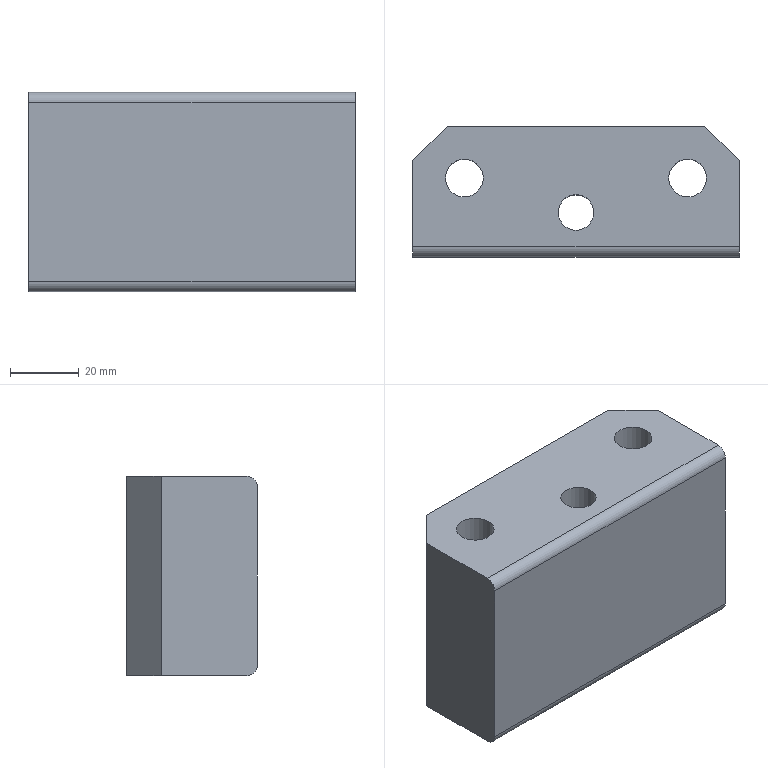Part | NX | features solid 2 | 1 solid | 19 faces | box 95 x 38 x 58 mm | volume 171870 mm3 | plane 11 | cylinder 8 | commonest cylinder face diameters 17 x3 6 x2 11 x2 10.3 x1
STEP:
#1=CARTESIAN_POINT('',(2412.5,497.,123.));
#2=VERTEX_POINT('',#1);
#3=CARTESIAN_POINT('',(2412.5,497.,71.));
#4=VERTEX_POINT('',#3);
#5=CARTESIAN_POINT('',(2412.5,497.,-60.));
#6=DIRECTION('',(0.,0.,-1.));
#7=VECTOR('',#6,1000.);
#8=LINE('',#5,#7);
#9=EDGE_CURVE('',#2,#4,#8,.T.);
#10=ORIENTED_EDGE('',*,*,#9,.T.);
#11=CARTESIAN_POINT('',(2507.5,497.,71.));
#12=VERTEX_POINT('',#11);
#13=CARTESIAN_POINT('',(2407.5,497.,71.));
#14=DIRECTION('',(1.,0.,0.));
#15=VECTOR('',#14,1000.);
#16=LINE('',#13,#15);
#17=EDGE_CURVE('',#4,#12,#16,.T.);
#18=ORIENTED_EDGE('',*,*,#17,.T.);
#19=CARTESIAN_POINT('',(2507.5,497.,123.));
#20=VERTEX_POINT('',#19);
#21=CARTESIAN_POINT('',(2507.5,497.,52.5));
#22=DIRECTION('',(0.,0.,1.));
#23=VECTOR('',#22,1000.);
#24=LINE('',#21,#23);
#25=EDGE_CURVE('',#12,#20,#24,.T.);
#26=ORIENTED_EDGE('',*,*,#25,.T.);
#27=CARTESIAN_POINT('',(2437.,497.,123.));
#28=DIRECTION('',(-1.,0.,0.));
#29=VECTOR('',#28,1000.);
#30=LINE('',#27,#29);
#31=EDGE_CURVE('',#20,#2,#30,.T.);
#32=ORIENTED_EDGE('',*,*,#31,.T.);
#33=EDGE_LOOP('',(#10,#18,#26,#32));
#34=FACE_BOUND('',#33,.T.);
#35=CARTESIAN_POINT('',(2437.,497.,99.));
#36=DIRECTION('',(0.,1.,0.));
#37=DIRECTION('',(0.,0.,1.));
#38=AXIS2_PLACEMENT_3D('',#35,#36,#37);
#39=PLANE('',#38);
#40=ADVANCED_FACE('',(#34),#39,.F.);
#41=CARTESIAN_POINT('',(2427.5,525.5,106.));
#42=VERTEX_POINT('',#41);
#43=CARTESIAN_POINT('',(2427.5,520.,106.));
#44=DIRECTION('',(0.,0.,-1.));
#45=DIRECTION('',(0.,1.,0.));
#46=AXIS2_PLACEMENT_3D('',#43,#44,#45);
#47=CIRCLE('',#46,5.5);
#48=EDGE_CURVE('',#42,#42,#47,.T.);
#49=ORIENTED_EDGE('',*,*,#48,.F.);
#50=EDGE_LOOP('',(#49));
#51=FACE_BOUND('',#50,.T.);
#52=CARTESIAN_POINT('',(2427.5,528.5,106.));
#53=VERTEX_POINT('',#52);
#54=CARTESIAN_POINT('',(2427.5,520.,106.));
#55=DIRECTION('',(0.,0.,-1.));
#56=DIRECTION('',(0.,1.,0.));
#57=AXIS2_PLACEMENT_3D('',#54,#55,#56);
#58=CIRCLE('',#57,8.5);
#59=EDGE_CURVE('',#53,#53,#58,.T.);
#60=ORIENTED_EDGE('',*,*,#59,.T.);
#61=EDGE_LOOP('',(#60));
#62=FACE_BOUND('',#61,.T.);
#63=CARTESIAN_POINT('',(1913.818,1175.578,106.));
#64=DIRECTION('',(0.,0.,1.));
#65=DIRECTION('',(0.,1.,0.));
#66=AXIS2_PLACEMENT_3D('',#63,#64,#65);
#67=PLANE('',#66);
#68=ADVANCED_FACE('',(#51,#62),#67,.F.);
#69=CARTESIAN_POINT('',(2492.5,525.5,106.));
#70=VERTEX_POINT('',#69);
#71=CARTESIAN_POINT('',(2492.5,520.,106.));
#72=DIRECTION('',(0.,0.,-1.));
#73=DIRECTION('',(0.,1.,0.));
#74=AXIS2_PLACEMENT_3D('',#71,#72,#73);
#75=CIRCLE('',#74,5.5);
#76=EDGE_CURVE('',#70,#70,#75,.T.);
#77=ORIENTED_EDGE('',*,*,#76,.F.);
#78=EDGE_LOOP('',(#77));
#79=FACE_BOUND('',#78,.T.);
#80=CARTESIAN_POINT('',(2492.5,528.5,106.));
#81=VERTEX_POINT('',#80);
#82=CARTESIAN_POINT('',(2492.5,520.,106.));
#83=DIRECTION('',(0.,0.,-1.));
#84=DIRECTION('',(0.,1.,0.));
#85=AXIS2_PLACEMENT_3D('',#82,#83,#84);
#86=CIRCLE('',#85,8.5);
#87=EDGE_CURVE('',#81,#81,#86,.T.);
#88=ORIENTED_EDGE('',*,*,#87,.T.);
#89=EDGE_LOOP('',(#88));
#90=FACE_BOUND('',#89,.T.);
#91=CARTESIAN_POINT('',(1906.818,1177.578,106.));
#92=DIRECTION('',(0.,0.,1.));
#93=DIRECTION('',(0.,1.,0.));
#94=AXIS2_PLACEMENT_3D('',#91,#92,#93);
#95=PLANE('',#94);
#96=ADVANCED_FACE('',(#79,#90),#95,.F.);
#97=CARTESIAN_POINT('',(2412.5,500.,68.));
#98=VERTEX_POINT('',#97);
#99=CARTESIAN_POINT('',(2412.5,500.,71.));
#100=DIRECTION('',(-1.,0.,0.));
#101=DIRECTION('',(0.,1.,0.));
#102=AXIS2_PLACEMENT_3D('',#99,#100,#101);
#103=CIRCLE('',#102,3.);
#104=EDGE_CURVE('',#98,#4,#103,.T.);
#105=ORIENTED_EDGE('',*,*,#104,.F.);
#106=CARTESIAN_POINT('',(2507.5,500.,68.));
#107=VERTEX_POINT('',#106);
#108=CARTESIAN_POINT('',(2467.5,500.,68.));
#109=DIRECTION('',(-1.,0.,0.));
#110=VECTOR('',#109,1000.);
#111=LINE('',#108,#110);
#112=EDGE_CURVE('',#107,#98,#111,.T.);
#113=ORIENTED_EDGE('',*,*,#112,.F.);
#114=CARTESIAN_POINT('',(2507.5,500.,71.));
#115=DIRECTION('',(-1.,0.,0.));
#116=DIRECTION('',(0.,0.,1.));
#117=AXIS2_PLACEMENT_3D('',#114,#115,#116);
#118=CIRCLE('',#117,3.);
#119=EDGE_CURVE('',#107,#12,#118,.T.);
#120=ORIENTED_EDGE('',*,*,#119,.T.);
#121=ORIENTED_EDGE('',*,*,#17,.F.);
#122=EDGE_LOOP('',(#105,#113,#120,#121));
#123=FACE_BOUND('',#122,.T.);
#124=CARTESIAN_POINT('',(1911.818,500.,71.));
#125=DIRECTION('',(1.,0.,0.));
#126=DIRECTION('',(0.,0.,1.));
#127=AXIS2_PLACEMENT_3D('',#124,#125,#126);
#128=CYLINDRICAL_SURFACE('',#127,3.);
#129=ADVANCED_FACE('',(#123),#128,.T.);
#130=CARTESIAN_POINT('',(2412.5,525.,68.));
#131=VERTEX_POINT('',#130);
#132=CARTESIAN_POINT('',(2412.5,390.,68.));
#133=DIRECTION('',(0.,-1.,0.));
#134=VECTOR('',#133,1000.);
#135=LINE('',#132,#134);
#136=EDGE_CURVE('',#131,#98,#135,.T.);
#137=ORIENTED_EDGE('',*,*,#136,.T.);
#138=ORIENTED_EDGE('',*,*,#104,.T.);
#139=ORIENTED_EDGE('',*,*,#9,.F.);
#140=CARTESIAN_POINT('',(2412.5,500.,126.));
#141=VERTEX_POINT('',#140);
#142=CARTESIAN_POINT('',(2412.5,500.,123.));
#143=DIRECTION('',(-1.,0.,0.));
#144=DIRECTION('',(0.,1.,0.));
#145=AXIS2_PLACEMENT_3D('',#142,#143,#144);
#146=CIRCLE('',#145,3.);
#147=EDGE_CURVE('',#2,#141,#146,.T.);
#148=ORIENTED_EDGE('',*,*,#147,.T.);
#149=CARTESIAN_POINT('',(2412.5,525.,126.));
#150=VERTEX_POINT('',#149);
#151=CARTESIAN_POINT('',(2412.5,390.,126.));
#152=DIRECTION('',(0.,1.,0.));
#153=VECTOR('',#152,1000.);
#154=LINE('',#151,#153);
#155=EDGE_CURVE('',#141,#150,#154,.T.);
#156=ORIENTED_EDGE('',*,*,#155,.T.);
#157=CARTESIAN_POINT('',(2412.5,525.,-60.));
#158=DIRECTION('',(0.,0.,-1.));
#159=VECTOR('',#158,1000.);
#160=LINE('',#157,#159);
#161=EDGE_CURVE('',#150,#131,#160,.T.);
#162=ORIENTED_EDGE('',*,*,#161,.T.);
#163=EDGE_LOOP('',(#137,#138,#139,#148,#156,#162));
#164=FACE_BOUND('',#163,.T.);
#165=CARTESIAN_POINT('',(2412.5,390.,-60.));
#166=DIRECTION('',(1.,0.,0.));
#167=DIRECTION('',(0.,1.,0.));
#168=AXIS2_PLACEMENT_3D('',#165,#166,#167);
#169=PLANE('',#168);
#170=ADVANCED_FACE('',(#164),#169,.F.);
#171=CARTESIAN_POINT('',(2422.5,535.,126.));
#172=VERTEX_POINT('',#171);
#173=CARTESIAN_POINT('',(2490.948,603.448,126.));
#174=DIRECTION('',(-0.7071,-0.7071,0.));
#175=VECTOR('',#174,1000.);
#176=LINE('',#173,#175);
#177=EDGE_CURVE('',#172,#150,#176,.T.);
#178=ORIENTED_EDGE('',*,*,#177,.F.);
#179=CARTESIAN_POINT('',(2422.5,535.,68.));
#180=VERTEX_POINT('',#179);
#181=CARTESIAN_POINT('',(2422.5,535.,52.5));
#182=DIRECTION('',(0.,0.,1.));
#183=VECTOR('',#182,1000.);
#184=LINE('',#181,#183);
#185=EDGE_CURVE('',#180,#172,#184,.T.);
#186=ORIENTED_EDGE('',*,*,#185,.F.);
#187=CARTESIAN_POINT('',(2490.948,603.448,68.));
#188=DIRECTION('',(0.7071,0.7071,0.));
#189=VECTOR('',#188,1000.);
#190=LINE('',#187,#189);
#191=EDGE_CURVE('',#131,#180,#190,.T.);
#192=ORIENTED_EDGE('',*,*,#191,.F.);
#193=ORIENTED_EDGE('',*,*,#161,.F.);
#194=EDGE_LOOP('',(#178,#186,#192,#193));
#195=FACE_BOUND('',#194,.T.);
#196=CARTESIAN_POINT('',(2422.5,535.,52.5));
#197=DIRECTION('',(-0.7071,0.7071,0.));
#198=DIRECTION('',(0.,0.,-1.));
#199=AXIS2_PLACEMENT_3D('',#196,#197,#198);
#200=PLANE('',#199);
#201=ADVANCED_FACE('',(#195),#200,.T.);
#202=CARTESIAN_POINT('',(2497.5,535.,126.));
#203=VERTEX_POINT('',#202);
#204=CARTESIAN_POINT('',(2435.,535.,126.));
#205=DIRECTION('',(1.,0.,0.));
#206=VECTOR('',#205,1000.);
#207=LINE('',#204,#206);
#208=EDGE_CURVE('',#172,#203,#207,.T.);
#209=ORIENTED_EDGE('',*,*,#208,.T.);
#210=CARTESIAN_POINT('',(2497.5,535.,68.));
#211=VERTEX_POINT('',#210);
#212=CARTESIAN_POINT('',(2497.5,535.,52.5));
#213=DIRECTION('',(0.,0.,-1.));
#214=VECTOR('',#213,1000.);
#215=LINE('',#212,#214);
#216=EDGE_CURVE('',#203,#211,#215,.T.);
#217=ORIENTED_EDGE('',*,*,#216,.T.);
#218=CARTESIAN_POINT('',(2435.,535.,68.));
#219=DIRECTION('',(-1.,0.,0.));
#220=VECTOR('',#219,1000.);
#221=LINE('',#218,#220);
#222=EDGE_CURVE('',#211,#180,#221,.T.);
#223=ORIENTED_EDGE('',*,*,#222,.T.);
#224=ORIENTED_EDGE('',*,*,#185,.T.);
#225=EDGE_LOOP('',(#209,#217,#223,#224));
#226=FACE_BOUND('',#225,.T.);
#227=CARTESIAN_POINT('',(2435.,535.,52.5));
#228=DIRECTION('',(0.,1.,0.));
#229=DIRECTION('',(0.,0.,1.));
#230=AXIS2_PLACEMENT_3D('',#227,#228,#229);
#231=PLANE('',#230);
#232=ADVANCED_FACE('',(#226),#231,.T.);
#233=CARTESIAN_POINT('',(2507.5,525.,126.));
#234=VERTEX_POINT('',#233);
#235=CARTESIAN_POINT('',(1880.87,1151.63,126.));
#236=DIRECTION('',(-0.7071,0.7071,0.));
#237=VECTOR('',#236,1000.);
#238=LINE('',#235,#237);
#239=EDGE_CURVE('',#234,#203,#238,.T.);
#240=ORIENTED_EDGE('',*,*,#239,.F.);
#241=CARTESIAN_POINT('',(2507.5,525.,68.));
#242=VERTEX_POINT('',#241);
#243=CARTESIAN_POINT('',(2507.5,525.,52.5));
#244=DIRECTION('',(0.,0.,1.));
#245=VECTOR('',#244,1000.);
#246=LINE('',#243,#245);
#247=EDGE_CURVE('',#242,#234,#246,.T.);
#248=ORIENTED_EDGE('',*,*,#247,.F.);
#249=CARTESIAN_POINT('',(1880.87,1151.63,68.));
#250=DIRECTION('',(0.7071,-0.7071,0.));
#251=VECTOR('',#250,1000.);
#252=LINE('',#249,#251);
#253=EDGE_CURVE('',#211,#242,#252,.T.);
#254=ORIENTED_EDGE('',*,*,#253,.F.);
#255=ORIENTED_EDGE('',*,*,#216,.F.);
#256=EDGE_LOOP('',(#240,#248,#254,#255));
#257=FACE_BOUND('',#256,.T.);
#258=CARTESIAN_POINT('',(2507.5,525.,52.5));
#259=DIRECTION('',(-0.7071,-0.7071,0.));
#260=DIRECTION('',(0.,0.,1.));
#261=AXIS2_PLACEMENT_3D('',#258,#259,#260);
#262=PLANE('',#261);
#263=ADVANCED_FACE('',(#257),#262,.F.);
#264=CARTESIAN_POINT('',(2507.5,500.,126.));
#265=VERTEX_POINT('',#264);
#266=CARTESIAN_POINT('',(2507.5,500.,123.));
#267=DIRECTION('',(1.,0.,0.));
#268=DIRECTION('',(0.,0.,1.));
#269=AXIS2_PLACEMENT_3D('',#266,#267,#268);
#270=CIRCLE('',#269,3.);
#271=EDGE_CURVE('',#265,#20,#270,.T.);
#272=ORIENTED_EDGE('',*,*,#271,.T.);
#273=ORIENTED_EDGE('',*,*,#25,.F.);
#274=ORIENTED_EDGE('',*,*,#119,.F.);
#275=CARTESIAN_POINT('',(2507.5,440.,68.));
#276=DIRECTION('',(0.,1.,0.));
#277=VECTOR('',#276,1000.);
#278=LINE('',#275,#277);
#279=EDGE_CURVE('',#107,#242,#278,.T.);
#280=ORIENTED_EDGE('',*,*,#279,.T.);
#281=ORIENTED_EDGE('',*,*,#247,.T.);
#282=CARTESIAN_POINT('',(2507.5,440.,126.));
#283=DIRECTION('',(0.,-1.,0.));
#284=VECTOR('',#283,1000.);
#285=LINE('',#282,#284);
#286=EDGE_CURVE('',#234,#265,#285,.T.);
#287=ORIENTED_EDGE('',*,*,#286,.T.);
#288=EDGE_LOOP('',(#272,#273,#274,#280,#281,#287));
#289=FACE_BOUND('',#288,.T.);
#290=CARTESIAN_POINT('',(2507.5,440.,52.5));
#291=DIRECTION('',(1.,0.,0.));
#292=DIRECTION('',(0.,0.,1.));
#293=AXIS2_PLACEMENT_3D('',#290,#291,#292);
#294=PLANE('',#293);
#295=ADVANCED_FACE('',(#289),#294,.T.);
#296=ORIENTED_EDGE('',*,*,#147,.F.);
#297=ORIENTED_EDGE('',*,*,#31,.F.);
#298=ORIENTED_EDGE('',*,*,#271,.F.);
#299=CARTESIAN_POINT('',(2407.5,500.,126.));
#300=DIRECTION('',(1.,0.,0.));
#301=VECTOR('',#300,1000.);
#302=LINE('',#299,#301);
#303=EDGE_CURVE('',#141,#265,#302,.T.);
#304=ORIENTED_EDGE('',*,*,#303,.F.);
#305=EDGE_LOOP('',(#296,#297,#298,#304));
#306=FACE_BOUND('',#305,.T.);
#307=CARTESIAN_POINT('',(2437.,500.,123.));
#308=DIRECTION('',(-1.,0.,0.));
#309=DIRECTION('',(0.,0.,-1.));
#310=AXIS2_PLACEMENT_3D('',#307,#308,#309);
#311=CYLINDRICAL_SURFACE('',#310,3.);
#312=ADVANCED_FACE('',(#306),#311,.T.);
#313=CARTESIAN_POINT('',(2427.5,525.5,126.));
#314=VERTEX_POINT('',#313);
#315=CARTESIAN_POINT('',(2427.5,520.,126.));
#316=DIRECTION('',(0.,0.,1.));
#317=DIRECTION('',(0.,1.,0.));
#318=AXIS2_PLACEMENT_3D('',#315,#316,#317);
#319=CIRCLE('',#318,5.5);
#320=EDGE_CURVE('',#314,#314,#319,.T.);
#321=ORIENTED_EDGE('',*,*,#320,.T.);
#322=EDGE_LOOP('',(#321));
#323=FACE_BOUND('',#322,.T.);
#324=ORIENTED_EDGE('',*,*,#48,.T.);
#325=EDGE_LOOP('',(#324));
#326=FACE_BOUND('',#325,.T.);
#327=CARTESIAN_POINT('',(2427.5,520.,566.));
#328=DIRECTION('',(0.,0.,1.));
#329=DIRECTION('',(0.,-1.,0.));
#330=AXIS2_PLACEMENT_3D('',#327,#328,#329);
#331=CYLINDRICAL_SURFACE('',#330,5.5);
#332=ADVANCED_FACE('',(#323,#326),#331,.F.);
#333=CARTESIAN_POINT('',(2492.5,525.5,126.));
#334=VERTEX_POINT('',#333);
#335=CARTESIAN_POINT('',(2492.5,520.,126.));
#336=DIRECTION('',(0.,0.,1.));
#337=DIRECTION('',(0.,1.,0.));
#338=AXIS2_PLACEMENT_3D('',#335,#336,#337);
#339=CIRCLE('',#338,5.5);
#340=EDGE_CURVE('',#334,#334,#339,.T.);
#341=ORIENTED_EDGE('',*,*,#340,.T.);
#342=EDGE_LOOP('',(#341));
#343=FACE_BOUND('',#342,.T.);
#344=ORIENTED_EDGE('',*,*,#76,.T.);
#345=EDGE_LOOP('',(#344));
#346=FACE_BOUND('',#345,.T.);
#347=CARTESIAN_POINT('',(2492.5,520.,566.));
#348=DIRECTION('',(0.,0.,1.));
#349=DIRECTION('',(0.,-1.,0.));
#350=AXIS2_PLACEMENT_3D('',#347,#348,#349);
#351=CYLINDRICAL_SURFACE('',#350,5.5);
#352=ADVANCED_FACE('',(#343,#346),#351,.F.);
#353=CARTESIAN_POINT('',(2454.85,510.,126.));
#354=VERTEX_POINT('',#353);
#355=CARTESIAN_POINT('',(2460.,510.,126.));
#356=DIRECTION('',(0.,0.,-1.));
#357=DIRECTION('',(-1.,0.,0.));
#358=AXIS2_PLACEMENT_3D('',#355,#356,#357);
#359=CIRCLE('',#358,5.15);
#360=EDGE_CURVE('',#354,#354,#359,.T.);
#361=ORIENTED_EDGE('',*,*,#360,.T.);
#362=EDGE_LOOP('',(#361));
#363=FACE_BOUND('',#362,.T.);
#364=ORIENTED_EDGE('',*,*,#340,.F.);
#365=EDGE_LOOP('',(#364));
#366=FACE_BOUND('',#365,.T.);
#367=ORIENTED_EDGE('',*,*,#320,.F.);
#368=EDGE_LOOP('',(#367));
#369=FACE_BOUND('',#368,.T.);
#370=ORIENTED_EDGE('',*,*,#303,.T.);
#371=ORIENTED_EDGE('',*,*,#286,.F.);
#372=ORIENTED_EDGE('',*,*,#239,.T.);
#373=ORIENTED_EDGE('',*,*,#208,.F.);
#374=ORIENTED_EDGE('',*,*,#177,.T.);
#375=ORIENTED_EDGE('',*,*,#155,.F.);
#376=EDGE_LOOP('',(#370,#371,#372,#373,#374,#375));
#377=FACE_BOUND('',#376,.T.);
#378=CARTESIAN_POINT('',(1911.818,1177.578,126.));
#379=DIRECTION('',(0.,0.,1.));
#380=DIRECTION('',(0.,1.,0.));
#381=AXIS2_PLACEMENT_3D('',#378,#379,#380);
#382=PLANE('',#381);
#383=ADVANCED_FACE('',(#363,#366,#369,#377),#382,.T.);
#384=ORIENTED_EDGE('',*,*,#59,.F.);
#385=EDGE_LOOP('',(#384));
#386=FACE_BOUND('',#385,.T.);
#387=CARTESIAN_POINT('',(2427.5,528.5,68.));
#388=VERTEX_POINT('',#387);
#389=CARTESIAN_POINT('',(2427.5,520.,68.));
#390=DIRECTION('',(0.,0.,1.));
#391=DIRECTION('',(0.,1.,0.));
#392=AXIS2_PLACEMENT_3D('',#389,#390,#391);
#393=CIRCLE('',#392,8.5);
#394=EDGE_CURVE('',#388,#388,#393,.T.);
#395=ORIENTED_EDGE('',*,*,#394,.F.);
#396=EDGE_LOOP('',(#395));
#397=FACE_BOUND('',#396,.T.);
#398=CARTESIAN_POINT('',(2427.5,520.,48.));
#399=DIRECTION('',(0.,0.,1.));
#400=DIRECTION('',(0.,-1.,0.));
#401=AXIS2_PLACEMENT_3D('',#398,#399,#400);
#402=CYLINDRICAL_SURFACE('',#401,8.5);
#403=ADVANCED_FACE('',(#386,#397),#402,.F.);
#404=ORIENTED_EDGE('',*,*,#87,.F.);
#405=EDGE_LOOP('',(#404));
#406=FACE_BOUND('',#405,.T.);
#407=CARTESIAN_POINT('',(2492.5,528.5,68.));
#408=VERTEX_POINT('',#407);
#409=CARTESIAN_POINT('',(2492.5,520.,68.));
#410=DIRECTION('',(0.,0.,1.));
#411=DIRECTION('',(0.,1.,0.));
#412=AXIS2_PLACEMENT_3D('',#409,#410,#411);
#413=CIRCLE('',#412,8.5);
#414=EDGE_CURVE('',#408,#408,#413,.T.);
#415=ORIENTED_EDGE('',*,*,#414,.F.);
#416=EDGE_LOOP('',(#415));
#417=FACE_BOUND('',#416,.T.);
#418=CARTESIAN_POINT('',(2492.5,520.,48.));
#419=DIRECTION('',(0.,0.,1.));
#420=DIRECTION('',(0.,-1.,0.));
#421=AXIS2_PLACEMENT_3D('',#418,#419,#420);
#422=CYLINDRICAL_SURFACE('',#421,8.5);
#423=ADVANCED_FACE('',(#406,#417),#422,.F.);
#424=CARTESIAN_POINT('',(2460.,518.5,68.));
#425=VERTEX_POINT('',#424);
#426=CARTESIAN_POINT('',(2460.,510.,68.));
#427=DIRECTION('',(0.,0.,1.));
#428=DIRECTION('',(0.,1.,0.));
#429=AXIS2_PLACEMENT_3D('',#426,#427,#428);
#430=CIRCLE('',#429,8.5);
#431=EDGE_CURVE('',#425,#425,#430,.T.);
#432=ORIENTED_EDGE('',*,*,#431,.T.);
#433=EDGE_LOOP('',(#432));
#434=FACE_BOUND('',#433,.T.);
#435=ORIENTED_EDGE('',*,*,#414,.T.);
#436=EDGE_LOOP('',(#435));
#437=FACE_BOUND('',#436,.T.);
#438=ORIENTED_EDGE('',*,*,#394,.T.);
#439=EDGE_LOOP('',(#438));
#440=FACE_BOUND('',#439,.T.);
#441=ORIENTED_EDGE('',*,*,#279,.F.);
#442=ORIENTED_EDGE('',*,*,#112,.T.);
#443=ORIENTED_EDGE('',*,*,#136,.F.);
#444=ORIENTED_EDGE('',*,*,#191,.T.);
#445=ORIENTED_EDGE('',*,*,#222,.F.);
#446=ORIENTED_EDGE('',*,*,#253,.T.);
#447=EDGE_LOOP('',(#441,#442,#443,#444,#445,#446));
#448=FACE_BOUND('',#447,.T.);
#449=CARTESIAN_POINT('',(1911.818,1177.578,68.));
#450=DIRECTION('',(0.,0.,1.));
#451=DIRECTION('',(0.,1.,0.));
#452=AXIS2_PLACEMENT_3D('',#449,#450,#451);
#453=PLANE('',#452);
#454=ADVANCED_FACE('',(#434,#437,#440,#448),#453,.F.);
#455=CARTESIAN_POINT('',(2454.85,510.,106.));
#456=VERTEX_POINT('',#455);
#457=CARTESIAN_POINT('',(2460.,510.,106.));
#458=DIRECTION('',(0.,0.,-1.));
#459=DIRECTION('',(-1.,0.,0.));
#460=AXIS2_PLACEMENT_3D('',#457,#458,#459);
#461=CIRCLE('',#460,5.15);
#462=EDGE_CURVE('',#456,#456,#461,.T.);
#463=ORIENTED_EDGE('',*,*,#462,.F.);
#464=EDGE_LOOP('',(#463));
#465=FACE_BOUND('',#464,.T.);
#466=CARTESIAN_POINT('',(2460.,518.5,106.));
#467=VERTEX_POINT('',#466);
#468=CARTESIAN_POINT('',(2460.,510.,106.));
#469=DIRECTION('',(0.,0.,-1.));
#470=DIRECTION('',(0.,1.,0.));
#471=AXIS2_PLACEMENT_3D('',#468,#469,#470);
#472=CIRCLE('',#471,8.5);
#473=EDGE_CURVE('',#467,#467,#472,.T.);
#474=ORIENTED_EDGE('',*,*,#473,.T.);
#475=EDGE_LOOP('',(#474));
#476=FACE_BOUND('',#475,.T.);
#477=CARTESIAN_POINT('',(1874.318,1167.578,106.));
#478=DIRECTION('',(0.,0.,1.));
#479=DIRECTION('',(0.,1.,0.));
#480=AXIS2_PLACEMENT_3D('',#477,#478,#479);
#481=PLANE('',#480);
#482=ADVANCED_FACE('',(#465,#476),#481,.F.);
#483=ORIENTED_EDGE('',*,*,#360,.F.);
#484=EDGE_LOOP('',(#483));
#485=FACE_BOUND('',#484,.T.);
#486=ORIENTED_EDGE('',*,*,#462,.T.);
#487=EDGE_LOOP('',(#486));
#488=FACE_BOUND('',#487,.T.);
#489=CARTESIAN_POINT('',(2460.,510.,566.));
#490=DIRECTION('',(0.,0.,1.));
#491=DIRECTION('',(0.,-1.,0.));
#492=AXIS2_PLACEMENT_3D('',#489,#490,#491);
#493=CYLINDRICAL_SURFACE('',#492,5.15);
#494=ADVANCED_FACE('',(#485,#488),#493,.F.);
#495=ORIENTED_EDGE('',*,*,#473,.F.);
#496=EDGE_LOOP('',(#495));
#497=FACE_BOUND('',#496,.T.);
#498=ORIENTED_EDGE('',*,*,#431,.F.);
#499=EDGE_LOOP('',(#498));
#500=FACE_BOUND('',#499,.T.);
#501=CARTESIAN_POINT('',(2460.,510.,48.));
#502=DIRECTION('',(0.,0.,1.));
#503=DIRECTION('',(0.,-1.,0.));
#504=AXIS2_PLACEMENT_3D('',#501,#502,#503);
#505=CYLINDRICAL_SURFACE('',#504,8.5);
#506=ADVANCED_FACE('',(#497,#500),#505,.F.);
#507=CLOSED_SHELL('',(#40,#68,#96,#129,#170,#201,#232,#263,#295,#312,#332,#352,#383,#403,#423,#454,#482,#494,#506));
#508=MANIFOLD_SOLID_BREP('',#507);
#509=(LENGTH_UNIT()NAMED_UNIT(*)SI_UNIT(.MILLI.,.METRE.));
#510=UNCERTAINTY_MEASURE_WITH_UNIT(LENGTH_MEASURE(0.00001),#509,'','');
#511=(NAMED_UNIT(*)PLANE_ANGLE_UNIT()SI_UNIT($,.RADIAN.));
#512=(NAMED_UNIT(*)SI_UNIT($,.STERADIAN.)SOLID_ANGLE_UNIT());
#513=(GEOMETRIC_REPRESENTATION_CONTEXT(3)GLOBAL_UNCERTAINTY_ASSIGNED_CONTEXT((#510))GLOBAL_UNIT_ASSIGNED_CONTEXT((#509,#511,#512))REPRESENTATION_CONTEXT('',''));
#514=ADVANCED_BREP_SHAPE_REPRESENTATION('',(#508),#513);